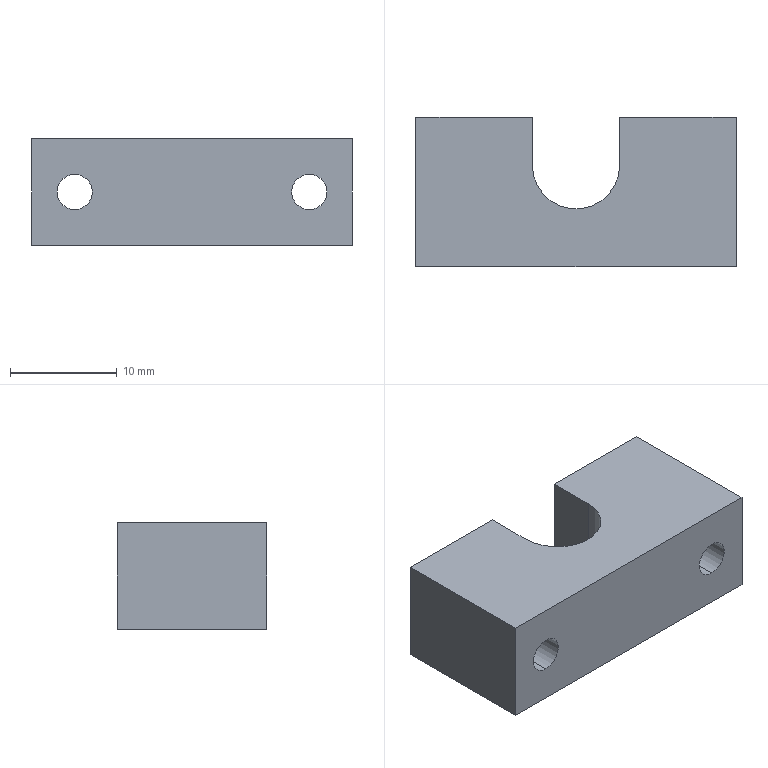Part | SolidWorks | features Extrusion 1, HoleWzd 1, ICE 1 | 1 solid | 14 faces | box 30 x 14 x 10 mm | volume 3327 mm3 | plane 9 | cylinder 5 | commonest cylinder face diameters 3.3 x4 8.2 x1
STEP:
#1=CARTESIAN_POINT('',(-11.,-7.,-1.65));
#2=VERTEX_POINT('',#1);
#3=CARTESIAN_POINT('',(-11.,-7.,1.65));
#4=VERTEX_POINT('',#3);
#5=CARTESIAN_POINT('',(-11.,-7.,0.));
#6=DIRECTION('',(0.,1.,0.));
#7=DIRECTION('',(0.,0.,1.));
#8=AXIS2_PLACEMENT_3D('',#5,#6,#7);
#9=CIRCLE('',#8,1.65);
#10=EDGE_CURVE('',#2,#4,#9,.T.);
#11=ORIENTED_EDGE('',*,*,#10,.F.);
#12=CARTESIAN_POINT('',(-11.,7.,-1.65));
#13=VERTEX_POINT('',#12);
#14=CARTESIAN_POINT('',(-11.,7.,-1.65));
#15=DIRECTION('',(0.,1.,0.));
#16=VECTOR('',#15,1000.);
#17=LINE('',#14,#16);
#18=EDGE_CURVE('',#2,#13,#17,.T.);
#19=ORIENTED_EDGE('',*,*,#18,.T.);
#20=CARTESIAN_POINT('',(-11.,7.,1.65));
#21=VERTEX_POINT('',#20);
#22=CARTESIAN_POINT('',(-11.,7.,0.));
#23=DIRECTION('',(0.,1.,0.));
#24=DIRECTION('',(0.,0.,1.));
#25=AXIS2_PLACEMENT_3D('',#22,#23,#24);
#26=CIRCLE('',#25,1.65);
#27=EDGE_CURVE('',#13,#21,#26,.T.);
#28=ORIENTED_EDGE('',*,*,#27,.T.);
#29=CARTESIAN_POINT('',(-11.,7.,1.65));
#30=DIRECTION('',(0.,1.,0.));
#31=VECTOR('',#30,1000.);
#32=LINE('',#29,#31);
#33=EDGE_CURVE('',#4,#21,#32,.T.);
#34=ORIENTED_EDGE('',*,*,#33,.F.);
#35=EDGE_LOOP('',(#11,#19,#28,#34));
#36=FACE_OUTER_BOUND('',#35,.T.);
#37=CARTESIAN_POINT('',(-11.,7.,0.));
#38=DIRECTION('',(0.,1.,0.));
#39=DIRECTION('',(0.,0.,1.));
#40=AXIS2_PLACEMENT_3D('',#37,#38,#39);
#41=CYLINDRICAL_SURFACE('',#40,1.65);
#42=ADVANCED_FACE('',(#36),#41,.F.);
#43=CARTESIAN_POINT('',(11.,-7.,-1.65));
#44=VERTEX_POINT('',#43);
#45=CARTESIAN_POINT('',(11.,-7.,1.65));
#46=VERTEX_POINT('',#45);
#47=CARTESIAN_POINT('',(11.,-7.,0.));
#48=DIRECTION('',(0.,1.,0.));
#49=DIRECTION('',(0.,0.,1.));
#50=AXIS2_PLACEMENT_3D('',#47,#48,#49);
#51=CIRCLE('',#50,1.65);
#52=EDGE_CURVE('',#44,#46,#51,.T.);
#53=ORIENTED_EDGE('',*,*,#52,.F.);
#54=CARTESIAN_POINT('',(11.,7.,-1.65));
#55=VERTEX_POINT('',#54);
#56=CARTESIAN_POINT('',(11.,7.,-1.65));
#57=DIRECTION('',(0.,1.,0.));
#58=VECTOR('',#57,1000.);
#59=LINE('',#56,#58);
#60=EDGE_CURVE('',#44,#55,#59,.T.);
#61=ORIENTED_EDGE('',*,*,#60,.T.);
#62=CARTESIAN_POINT('',(11.,7.,1.65));
#63=VERTEX_POINT('',#62);
#64=CARTESIAN_POINT('',(11.,7.,0.));
#65=DIRECTION('',(0.,1.,0.));
#66=DIRECTION('',(0.,0.,1.));
#67=AXIS2_PLACEMENT_3D('',#64,#65,#66);
#68=CIRCLE('',#67,1.65);
#69=EDGE_CURVE('',#55,#63,#68,.T.);
#70=ORIENTED_EDGE('',*,*,#69,.T.);
#71=CARTESIAN_POINT('',(11.,7.,1.65));
#72=DIRECTION('',(0.,1.,0.));
#73=VECTOR('',#72,1000.);
#74=LINE('',#71,#73);
#75=EDGE_CURVE('',#46,#63,#74,.T.);
#76=ORIENTED_EDGE('',*,*,#75,.F.);
#77=EDGE_LOOP('',(#53,#61,#70,#76));
#78=FACE_OUTER_BOUND('',#77,.T.);
#79=CARTESIAN_POINT('',(11.,7.,0.));
#80=DIRECTION('',(0.,1.,0.));
#81=DIRECTION('',(0.,0.,1.));
#82=AXIS2_PLACEMENT_3D('',#79,#80,#81);
#83=CYLINDRICAL_SURFACE('',#82,1.65);
#84=ADVANCED_FACE('',(#78),#83,.F.);
#85=CARTESIAN_POINT('',(11.,7.,0.));
#86=DIRECTION('',(0.,1.,0.));
#87=DIRECTION('',(0.,0.,1.));
#88=AXIS2_PLACEMENT_3D('',#85,#86,#87);
#89=CIRCLE('',#88,1.65);
#90=EDGE_CURVE('',#63,#55,#89,.T.);
#91=ORIENTED_EDGE('',*,*,#90,.F.);
#92=ORIENTED_EDGE('',*,*,#69,.F.);
#93=EDGE_LOOP('',(#91,#92));
#94=FACE_BOUND('',#93,.T.);
#95=CARTESIAN_POINT('',(15.,7.,-5.));
#96=VERTEX_POINT('',#95);
#97=CARTESIAN_POINT('',(4.1,7.,-5.));
#98=VERTEX_POINT('',#97);
#99=CARTESIAN_POINT('',(-15.,7.,-5.));
#100=DIRECTION('',(-1.,0.,0.));
#101=VECTOR('',#100,1000.);
#102=LINE('',#99,#101);
#103=EDGE_CURVE('',#96,#98,#102,.T.);
#104=ORIENTED_EDGE('',*,*,#103,.T.);
#105=CARTESIAN_POINT('',(4.1,7.,5.));
#106=VERTEX_POINT('',#105);
#107=CARTESIAN_POINT('',(4.1,7.,-5.));
#108=DIRECTION('',(0.,0.,1.));
#109=VECTOR('',#108,1000.);
#110=LINE('',#107,#109);
#111=EDGE_CURVE('',#98,#106,#110,.T.);
#112=ORIENTED_EDGE('',*,*,#111,.T.);
#113=CARTESIAN_POINT('',(15.,7.,5.));
#114=VERTEX_POINT('',#113);
#115=CARTESIAN_POINT('',(-15.,7.,5.));
#116=DIRECTION('',(-1.,0.,0.));
#117=VECTOR('',#116,1000.);
#118=LINE('',#115,#117);
#119=EDGE_CURVE('',#114,#106,#118,.T.);
#120=ORIENTED_EDGE('',*,*,#119,.F.);
#121=CARTESIAN_POINT('',(15.,7.,5.));
#122=DIRECTION('',(0.,0.,-1.));
#123=VECTOR('',#122,1000.);
#124=LINE('',#121,#123);
#125=EDGE_CURVE('',#114,#96,#124,.T.);
#126=ORIENTED_EDGE('',*,*,#125,.T.);
#127=EDGE_LOOP('',(#104,#112,#120,#126));
#128=FACE_OUTER_BOUND('',#127,.T.);
#129=CARTESIAN_POINT('',(-15.,7.,5.));
#130=DIRECTION('',(0.,-1.,0.));
#131=DIRECTION('',(0.,0.,-1.));
#132=AXIS2_PLACEMENT_3D('',#129,#130,#131);
#133=PLANE('',#132);
#134=ADVANCED_FACE('',(#94,#128),#133,.F.);
#135=CARTESIAN_POINT('',(15.,-7.,-5.));
#136=VERTEX_POINT('',#135);
#137=CARTESIAN_POINT('',(15.,7.,-5.));
#138=DIRECTION('',(0.,1.,0.));
#139=VECTOR('',#138,1000.);
#140=LINE('',#137,#139);
#141=EDGE_CURVE('',#136,#96,#140,.T.);
#142=ORIENTED_EDGE('',*,*,#141,.T.);
#143=ORIENTED_EDGE('',*,*,#125,.F.);
#144=CARTESIAN_POINT('',(15.,-7.,5.));
#145=VERTEX_POINT('',#144);
#146=CARTESIAN_POINT('',(15.,7.,5.));
#147=DIRECTION('',(0.,1.,0.));
#148=VECTOR('',#147,1000.);
#149=LINE('',#146,#148);
#150=EDGE_CURVE('',#145,#114,#149,.T.);
#151=ORIENTED_EDGE('',*,*,#150,.F.);
#152=CARTESIAN_POINT('',(15.,-7.,5.));
#153=DIRECTION('',(0.,0.,-1.));
#154=VECTOR('',#153,1000.);
#155=LINE('',#152,#154);
#156=EDGE_CURVE('',#145,#136,#155,.T.);
#157=ORIENTED_EDGE('',*,*,#156,.T.);
#158=EDGE_LOOP('',(#142,#143,#151,#157));
#159=FACE_OUTER_BOUND('',#158,.T.);
#160=CARTESIAN_POINT('',(15.,7.,5.));
#161=DIRECTION('',(-1.,0.,0.));
#162=DIRECTION('',(0.,-1.,0.));
#163=AXIS2_PLACEMENT_3D('',#160,#161,#162);
#164=PLANE('',#163);
#165=ADVANCED_FACE('',(#159),#164,.F.);
#166=CARTESIAN_POINT('',(-11.,7.,0.));
#167=DIRECTION('',(0.,1.,0.));
#168=DIRECTION('',(0.,0.,1.));
#169=AXIS2_PLACEMENT_3D('',#166,#167,#168);
#170=CIRCLE('',#169,1.65);
#171=EDGE_CURVE('',#21,#13,#170,.T.);
#172=ORIENTED_EDGE('',*,*,#171,.F.);
#173=ORIENTED_EDGE('',*,*,#27,.F.);
#174=EDGE_LOOP('',(#172,#173));
#175=FACE_BOUND('',#174,.T.);
#176=CARTESIAN_POINT('',(-4.1,7.,5.));
#177=VERTEX_POINT('',#176);
#178=CARTESIAN_POINT('',(-15.,7.,5.));
#179=VERTEX_POINT('',#178);
#180=CARTESIAN_POINT('',(-15.,7.,5.));
#181=DIRECTION('',(-1.,0.,0.));
#182=VECTOR('',#181,1000.);
#183=LINE('',#180,#182);
#184=EDGE_CURVE('',#177,#179,#183,.T.);
#185=ORIENTED_EDGE('',*,*,#184,.F.);
#186=CARTESIAN_POINT('',(-4.1,7.,-5.));
#187=VERTEX_POINT('',#186);
#188=CARTESIAN_POINT('',(-4.1,7.,-5.));
#189=DIRECTION('',(0.,0.,1.));
#190=VECTOR('',#189,1000.);
#191=LINE('',#188,#190);
#192=EDGE_CURVE('',#187,#177,#191,.T.);
#193=ORIENTED_EDGE('',*,*,#192,.F.);
#194=CARTESIAN_POINT('',(-15.,7.,-5.));
#195=VERTEX_POINT('',#194);
#196=CARTESIAN_POINT('',(-15.,7.,-5.));
#197=DIRECTION('',(-1.,0.,0.));
#198=VECTOR('',#197,1000.);
#199=LINE('',#196,#198);
#200=EDGE_CURVE('',#187,#195,#199,.T.);
#201=ORIENTED_EDGE('',*,*,#200,.T.);
#202=CARTESIAN_POINT('',(-15.,7.,5.));
#203=DIRECTION('',(0.,0.,-1.));
#204=VECTOR('',#203,1000.);
#205=LINE('',#202,#204);
#206=EDGE_CURVE('',#179,#195,#205,.T.);
#207=ORIENTED_EDGE('',*,*,#206,.F.);
#208=EDGE_LOOP('',(#185,#193,#201,#207));
#209=FACE_OUTER_BOUND('',#208,.T.);
#210=CARTESIAN_POINT('',(-15.,7.,5.));
#211=DIRECTION('',(0.,-1.,0.));
#212=DIRECTION('',(0.,0.,-1.));
#213=AXIS2_PLACEMENT_3D('',#210,#211,#212);
#214=PLANE('',#213);
#215=ADVANCED_FACE('',(#175,#209),#214,.F.);
#216=CARTESIAN_POINT('',(-15.,-7.,-5.));
#217=VERTEX_POINT('',#216);
#218=CARTESIAN_POINT('',(-15.,7.,-5.));
#219=DIRECTION('',(0.,-1.,0.));
#220=VECTOR('',#219,1000.);
#221=LINE('',#218,#220);
#222=EDGE_CURVE('',#195,#217,#221,.T.);
#223=ORIENTED_EDGE('',*,*,#222,.T.);
#224=CARTESIAN_POINT('',(-15.,-7.,5.));
#225=VERTEX_POINT('',#224);
#226=CARTESIAN_POINT('',(-15.,-7.,5.));
#227=DIRECTION('',(0.,0.,-1.));
#228=VECTOR('',#227,1000.);
#229=LINE('',#226,#228);
#230=EDGE_CURVE('',#225,#217,#229,.T.);
#231=ORIENTED_EDGE('',*,*,#230,.F.);
#232=CARTESIAN_POINT('',(-15.,7.,5.));
#233=DIRECTION('',(0.,-1.,0.));
#234=VECTOR('',#233,1000.);
#235=LINE('',#232,#234);
#236=EDGE_CURVE('',#179,#225,#235,.T.);
#237=ORIENTED_EDGE('',*,*,#236,.F.);
#238=ORIENTED_EDGE('',*,*,#206,.T.);
#239=EDGE_LOOP('',(#223,#231,#237,#238));
#240=FACE_OUTER_BOUND('',#239,.T.);
#241=CARTESIAN_POINT('',(-15.,7.,5.));
#242=DIRECTION('',(1.,0.,0.));
#243=DIRECTION('',(0.,1.,0.));
#244=AXIS2_PLACEMENT_3D('',#241,#242,#243);
#245=PLANE('',#244);
#246=ADVANCED_FACE('',(#240),#245,.F.);
#247=CARTESIAN_POINT('',(-11.,-7.,0.));
#248=DIRECTION('',(0.,1.,0.));
#249=DIRECTION('',(0.,0.,1.));
#250=AXIS2_PLACEMENT_3D('',#247,#248,#249);
#251=CIRCLE('',#250,1.65);
#252=EDGE_CURVE('',#4,#2,#251,.T.);
#253=ORIENTED_EDGE('',*,*,#252,.T.);
#254=ORIENTED_EDGE('',*,*,#10,.T.);
#255=EDGE_LOOP('',(#253,#254));
#256=FACE_BOUND('',#255,.T.);
#257=CARTESIAN_POINT('',(11.,-7.,0.));
#258=DIRECTION('',(0.,1.,0.));
#259=DIRECTION('',(0.,0.,1.));
#260=AXIS2_PLACEMENT_3D('',#257,#258,#259);
#261=CIRCLE('',#260,1.65);
#262=EDGE_CURVE('',#46,#44,#261,.T.);
#263=ORIENTED_EDGE('',*,*,#262,.T.);
#264=ORIENTED_EDGE('',*,*,#52,.T.);
#265=EDGE_LOOP('',(#263,#264));
#266=FACE_BOUND('',#265,.T.);
#267=CARTESIAN_POINT('',(-15.,-7.,-5.));
#268=DIRECTION('',(1.,0.,0.));
#269=VECTOR('',#268,1000.);
#270=LINE('',#267,#269);
#271=EDGE_CURVE('',#217,#136,#270,.T.);
#272=ORIENTED_EDGE('',*,*,#271,.T.);
#273=ORIENTED_EDGE('',*,*,#156,.F.);
#274=CARTESIAN_POINT('',(-15.,-7.,5.));
#275=DIRECTION('',(1.,0.,0.));
#276=VECTOR('',#275,1000.);
#277=LINE('',#274,#276);
#278=EDGE_CURVE('',#225,#145,#277,.T.);
#279=ORIENTED_EDGE('',*,*,#278,.F.);
#280=ORIENTED_EDGE('',*,*,#230,.T.);
#281=EDGE_LOOP('',(#272,#273,#279,#280));
#282=FACE_OUTER_BOUND('',#281,.T.);
#283=CARTESIAN_POINT('',(-15.,-7.,5.));
#284=DIRECTION('',(0.,1.,0.));
#285=DIRECTION('',(0.,0.,1.));
#286=AXIS2_PLACEMENT_3D('',#283,#284,#285);
#287=PLANE('',#286);
#288=ADVANCED_FACE('',(#256,#266,#282),#287,.F.);
#289=CARTESIAN_POINT('',(4.1,2.5,5.));
#290=VERTEX_POINT('',#289);
#291=CARTESIAN_POINT('',(4.1,7.,5.));
#292=DIRECTION('',(0.,1.,0.));
#293=VECTOR('',#292,1000.);
#294=LINE('',#291,#293);
#295=EDGE_CURVE('',#290,#106,#294,.T.);
#296=ORIENTED_EDGE('',*,*,#295,.F.);
#297=CARTESIAN_POINT('',(-4.1,2.5,5.));
#298=VERTEX_POINT('',#297);
#299=CARTESIAN_POINT('',(0.,2.5,5.));
#300=DIRECTION('',(0.,0.,1.));
#301=DIRECTION('',(1.,0.,0.));
#302=AXIS2_PLACEMENT_3D('',#299,#300,#301);
#303=CIRCLE('',#302,4.1);
#304=EDGE_CURVE('',#298,#290,#303,.T.);
#305=ORIENTED_EDGE('',*,*,#304,.F.);
#306=CARTESIAN_POINT('',(-4.1,7.,5.));
#307=DIRECTION('',(0.,-1.,0.));
#308=VECTOR('',#307,1000.);
#309=LINE('',#306,#308);
#310=EDGE_CURVE('',#177,#298,#309,.T.);
#311=ORIENTED_EDGE('',*,*,#310,.F.);
#312=ORIENTED_EDGE('',*,*,#184,.T.);
#313=ORIENTED_EDGE('',*,*,#236,.T.);
#314=ORIENTED_EDGE('',*,*,#278,.T.);
#315=ORIENTED_EDGE('',*,*,#150,.T.);
#316=ORIENTED_EDGE('',*,*,#119,.T.);
#317=EDGE_LOOP('',(#296,#305,#311,#312,#313,#314,#315,#316));
#318=FACE_OUTER_BOUND('',#317,.T.);
#319=CARTESIAN_POINT('',(0.,0.,5.));
#320=DIRECTION('',(0.,0.,1.));
#321=DIRECTION('',(1.,0.,0.));
#322=AXIS2_PLACEMENT_3D('',#319,#320,#321);
#323=PLANE('',#322);
#324=ADVANCED_FACE('',(#318),#323,.T.);
#325=CARTESIAN_POINT('',(-4.1,2.5,-5.));
#326=VERTEX_POINT('',#325);
#327=CARTESIAN_POINT('',(4.1,2.5,-5.));
#328=VERTEX_POINT('',#327);
#329=CARTESIAN_POINT('',(0.,2.5,-5.));
#330=DIRECTION('',(0.,0.,1.));
#331=DIRECTION('',(1.,0.,0.));
#332=AXIS2_PLACEMENT_3D('',#329,#330,#331);
#333=CIRCLE('',#332,4.1);
#334=EDGE_CURVE('',#326,#328,#333,.T.);
#335=ORIENTED_EDGE('',*,*,#334,.T.);
#336=CARTESIAN_POINT('',(4.1,7.,-5.));
#337=DIRECTION('',(0.,1.,0.));
#338=VECTOR('',#337,1000.);
#339=LINE('',#336,#338);
#340=EDGE_CURVE('',#328,#98,#339,.T.);
#341=ORIENTED_EDGE('',*,*,#340,.T.);
#342=ORIENTED_EDGE('',*,*,#103,.F.);
#343=ORIENTED_EDGE('',*,*,#141,.F.);
#344=ORIENTED_EDGE('',*,*,#271,.F.);
#345=ORIENTED_EDGE('',*,*,#222,.F.);
#346=ORIENTED_EDGE('',*,*,#200,.F.);
#347=CARTESIAN_POINT('',(-4.1,7.,-5.));
#348=DIRECTION('',(0.,-1.,0.));
#349=VECTOR('',#348,1000.);
#350=LINE('',#347,#349);
#351=EDGE_CURVE('',#187,#326,#350,.T.);
#352=ORIENTED_EDGE('',*,*,#351,.T.);
#353=EDGE_LOOP('',(#335,#341,#342,#343,#344,#345,#346,#352));
#354=FACE_OUTER_BOUND('',#353,.T.);
#355=CARTESIAN_POINT('',(0.,0.,-5.));
#356=DIRECTION('',(0.,0.,1.));
#357=DIRECTION('',(1.,0.,0.));
#358=AXIS2_PLACEMENT_3D('',#355,#356,#357);
#359=PLANE('',#358);
#360=ADVANCED_FACE('',(#354),#359,.F.);
#361=ORIENTED_EDGE('',*,*,#295,.T.);
#362=ORIENTED_EDGE('',*,*,#111,.F.);
#363=ORIENTED_EDGE('',*,*,#340,.F.);
#364=CARTESIAN_POINT('',(4.1,2.5,-5.));
#365=DIRECTION('',(0.,0.,1.));
#366=VECTOR('',#365,1000.);
#367=LINE('',#364,#366);
#368=EDGE_CURVE('',#328,#290,#367,.T.);
#369=ORIENTED_EDGE('',*,*,#368,.T.);
#370=EDGE_LOOP('',(#361,#362,#363,#369));
#371=FACE_OUTER_BOUND('',#370,.T.);
#372=CARTESIAN_POINT('',(4.1,7.,-5.));
#373=DIRECTION('',(1.,0.,0.));
#374=DIRECTION('',(0.,1.,0.));
#375=AXIS2_PLACEMENT_3D('',#372,#373,#374);
#376=PLANE('',#375);
#377=ADVANCED_FACE('',(#371),#376,.F.);
#378=ORIENTED_EDGE('',*,*,#304,.T.);
#379=ORIENTED_EDGE('',*,*,#368,.F.);
#380=ORIENTED_EDGE('',*,*,#334,.F.);
#381=CARTESIAN_POINT('',(-4.1,2.5,-5.));
#382=DIRECTION('',(0.,0.,1.));
#383=VECTOR('',#382,1000.);
#384=LINE('',#381,#383);
#385=EDGE_CURVE('',#326,#298,#384,.T.);
#386=ORIENTED_EDGE('',*,*,#385,.T.);
#387=EDGE_LOOP('',(#378,#379,#380,#386));
#388=FACE_OUTER_BOUND('',#387,.T.);
#389=CARTESIAN_POINT('',(0.,2.5,-5.));
#390=DIRECTION('',(0.,0.,1.));
#391=DIRECTION('',(1.,0.,0.));
#392=AXIS2_PLACEMENT_3D('',#389,#390,#391);
#393=CYLINDRICAL_SURFACE('',#392,4.1);
#394=ADVANCED_FACE('',(#388),#393,.F.);
#395=ORIENTED_EDGE('',*,*,#310,.T.);
#396=ORIENTED_EDGE('',*,*,#385,.F.);
#397=ORIENTED_EDGE('',*,*,#351,.F.);
#398=ORIENTED_EDGE('',*,*,#192,.T.);
#399=EDGE_LOOP('',(#395,#396,#397,#398));
#400=FACE_OUTER_BOUND('',#399,.T.);
#401=CARTESIAN_POINT('',(-4.1,7.,-5.));
#402=DIRECTION('',(-1.,0.,0.));
#403=DIRECTION('',(0.,-1.,0.));
#404=AXIS2_PLACEMENT_3D('',#401,#402,#403);
#405=PLANE('',#404);
#406=ADVANCED_FACE('',(#400),#405,.F.);
#407=ORIENTED_EDGE('',*,*,#60,.F.);
#408=ORIENTED_EDGE('',*,*,#262,.F.);
#409=ORIENTED_EDGE('',*,*,#75,.T.);
#410=ORIENTED_EDGE('',*,*,#90,.T.);
#411=EDGE_LOOP('',(#407,#408,#409,#410));
#412=FACE_OUTER_BOUND('',#411,.T.);
#413=CARTESIAN_POINT('',(11.,7.,0.));
#414=DIRECTION('',(0.,1.,0.));
#415=DIRECTION('',(0.,0.,1.));
#416=AXIS2_PLACEMENT_3D('',#413,#414,#415);
#417=CYLINDRICAL_SURFACE('',#416,1.65);
#418=ADVANCED_FACE('',(#412),#417,.F.);
#419=ORIENTED_EDGE('',*,*,#18,.F.);
#420=ORIENTED_EDGE('',*,*,#252,.F.);
#421=ORIENTED_EDGE('',*,*,#33,.T.);
#422=ORIENTED_EDGE('',*,*,#171,.T.);
#423=EDGE_LOOP('',(#419,#420,#421,#422));
#424=FACE_OUTER_BOUND('',#423,.T.);
#425=CARTESIAN_POINT('',(-11.,7.,0.));
#426=DIRECTION('',(0.,1.,0.));
#427=DIRECTION('',(0.,0.,1.));
#428=AXIS2_PLACEMENT_3D('',#425,#426,#427);
#429=CYLINDRICAL_SURFACE('',#428,1.65);
#430=ADVANCED_FACE('',(#424),#429,.F.);
#431=CLOSED_SHELL('',(#42,#84,#134,#165,#215,#246,#288,#324,#360,#377,#394,#406,#418,#430));
#432=MANIFOLD_SOLID_BREP('',#431);
#433=CARTESIAN_POINT('',(0.,0.,0.));
#434=DIRECTION('',(0.,0.,1.));
#435=DIRECTION('',(1.,0.,0.));
#436=AXIS2_PLACEMENT_3D('',#433,#434,#435);
#437=(LENGTH_UNIT()NAMED_UNIT(*)SI_UNIT(.MILLI.,.METRE.));
#438=UNCERTAINTY_MEASURE_WITH_UNIT(LENGTH_MEASURE(0.00001),#437,'','');
#439=(NAMED_UNIT(*)PLANE_ANGLE_UNIT()SI_UNIT($,.RADIAN.));
#440=(NAMED_UNIT(*)SI_UNIT($,.STERADIAN.)SOLID_ANGLE_UNIT());
#441=(GEOMETRIC_REPRESENTATION_CONTEXT(3)GLOBAL_UNCERTAINTY_ASSIGNED_CONTEXT((#438))GLOBAL_UNIT_ASSIGNED_CONTEXT((#437,#439,#440))REPRESENTATION_CONTEXT('',''));
#442=ADVANCED_BREP_SHAPE_REPRESENTATION('',(#432,#436),#441);